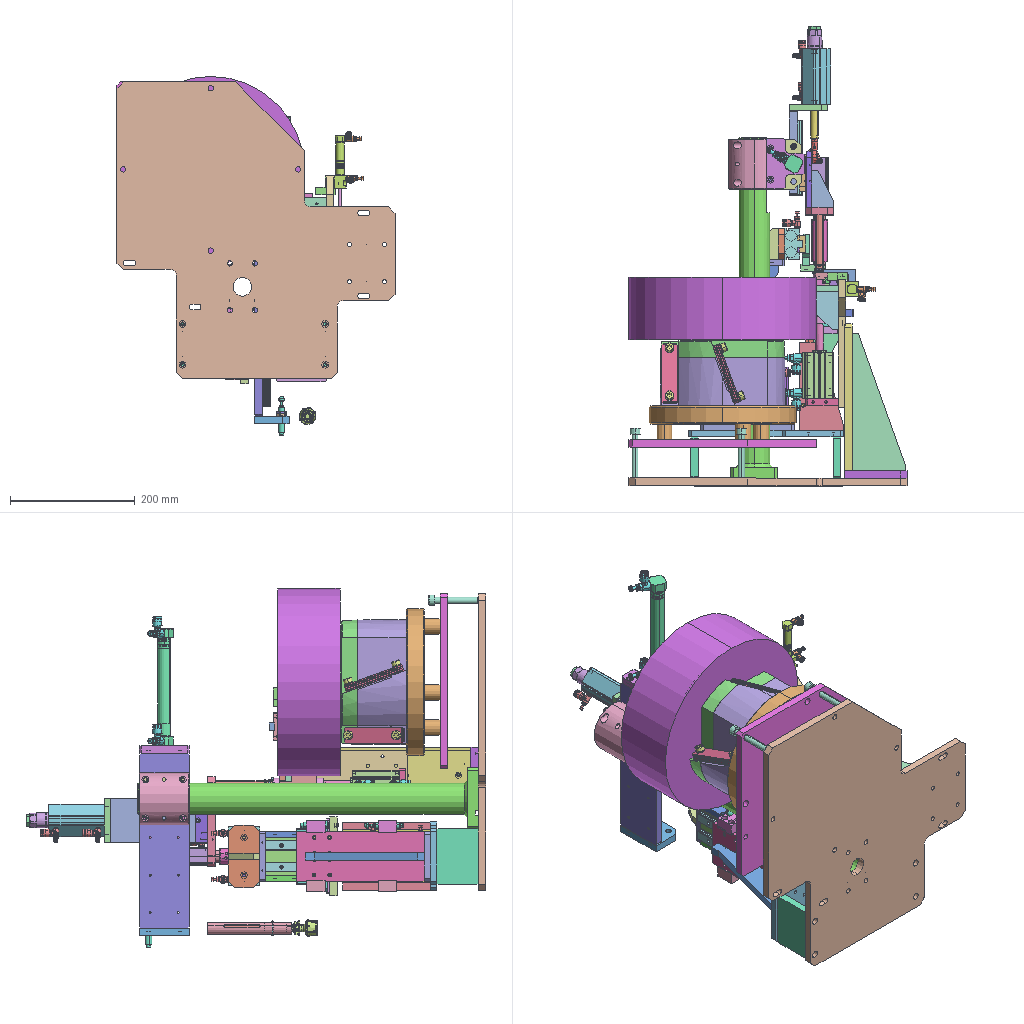Assembly | STEP file | 112 different items | 228 placed | box 445 x 736 x 575 mm
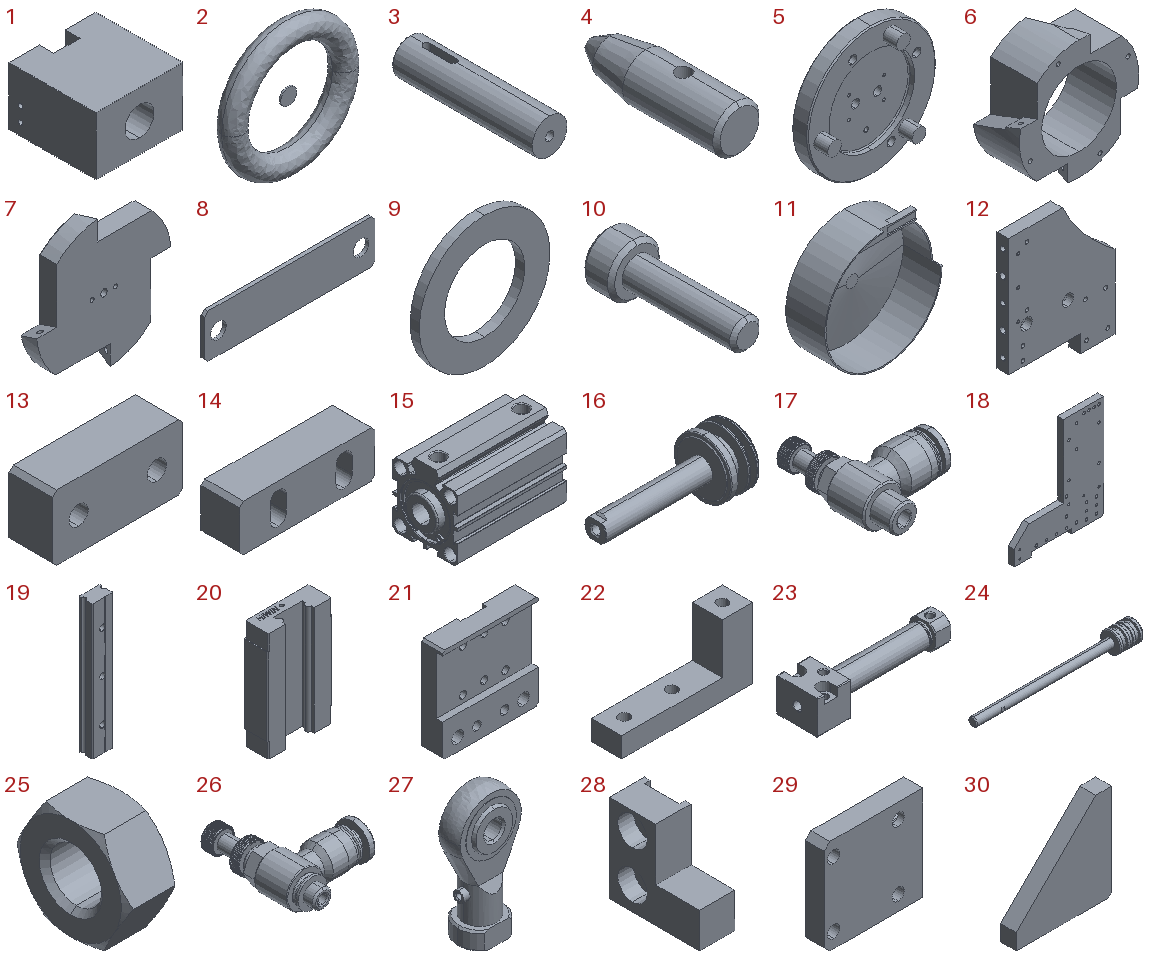Parts list (item | name | quantity | parent item | size | volume):
1 | PN_0053 | x1 | in PN_0052 | 60 x 60 x 40 mm | 121912 mm3
2 | 20501 | x14 | in PN_0052, PN_0061 | 16.4 x 2.7 x 16.4 mm | 247.033 mm3
3 | PN_0054 | x1 | in PN_0052 | 20 x 80 x 20 mm | 15788 mm3
4 | PN_0055 | x1 | in PN_0052 | 12.5 x 40 x 12.5 mm | 3984 mm3
5 | Vibration plate 3-04_default | x1 | in Vibration plate 3-02_default | 235 x 74 x 235 mm | 1320823 mm3
6 | Vibration plate 3-03_default | x1 | in Vibration plate 3-02_default | 200 x 78 x 200 mm | 1058700 mm3
7 | Vibration plate 3-08_default | x2 | in Vibration plate 3-02_default | 199.095 x 28 x 199.095 mm | 629211 mm3
8 | Vibration plate 3-07_default | x16 | in Vibration plate 3-02_default | 98 x 2 x 25 mm | 4630 mm3
9 | Vibration plate 3-06_default | x32 | in Vibration plate 3-02_default | 14 x 1 x 14 mm | 95.85 mm3
10 | Vibration plate 3-05_default | x12 | in Vibration plate 3-02_default | 14 x 38 x 14 mm | 2499 mm3
11 | Vibration plate 20501 | x1 | in Vibration plate 20501_default | 300 x 100 x 300 mm | 987568 mm3
12 | PN_0003 | x1 | in PN_0052 | 90 x 10 x 115 mm | 78081 mm3
13 | PN_0004 | x1 | in PN_0052 | 30 x 10 x 15 mm | 4176 mm3
14 | PN_0005 | x1 | in PN_0052 | 35 x 10 x 12 mm | 3567 mm3
15 | SDA32x40S-01-cc | x1 | in SDA32x40S-cc | 77.5 x 44 x 50 mm | 81433 mm3
16 | SDA32x40S-02-cc | x1 | in SDA32x40S-cc | 75.5 x 31.9 x 31.9 mm | 15906 mm3
17 | PSL801A | x4 | in SDA32x40S-cc, MI20x125SU-cc | 33.8 x 41.6 x 14.7 mm | 5385 mm3
18 | PN_0006 | x1 | in PN_0052 | 179.5 x 12 x 205 mm | 243420 mm3
19 | MGN12H-80-01-CC | x1 | in MGN12H-80-CC | 12 x 8 x 80 mm | 6824 mm3
20 | MGN12H-80-02-CC | x1 | in MGN12H-80-CC | 27 x 10 x 45.4 mm | 9266 mm3
21 | PN_0007 | x1 | in PN_0052 | 45 x 10 x 44.5 mm | 13324 mm3
22 | PN_0008 | x1 | in PN_0052 | 52 x 12 x 28 mm | 7462 mm3
23 | PBR12X30SU-01-CC | x1 | in PBR12X30SU-CC | 84 x 24.2 x 20 mm | 10911 mm3
24 | PBR12X30SU-02-CC | x1 | in PBR12X30SU-CC | 94.5 x 12 x 12 mm | 2851 mm3
25 | PBR12X30SU-03-CC | x1 | in PBR12X30SU-CC | 4 x 9.238 x 8 mm | 164.283 mm3
26 | PSL4M5A | x2 | in PBR12X30SU-CC | 23.8 x 30 x 9.8 mm | 1827 mm3
27 | F-M5X080U | x1 | in PBR12X30SU-CC | - | 2766 mm3
28 | PN_0009 | x1 | in PN_0052 | 12 x 31 x 30 mm | 6133 mm3
29 | PN_0010 | x1 | in PN_0052 | 52 x 10 x 50 mm | 23516 mm3
30 | PN_0011 | x1 | in PN_0052 | 60 x 10 x 60 mm | 22770 mm3
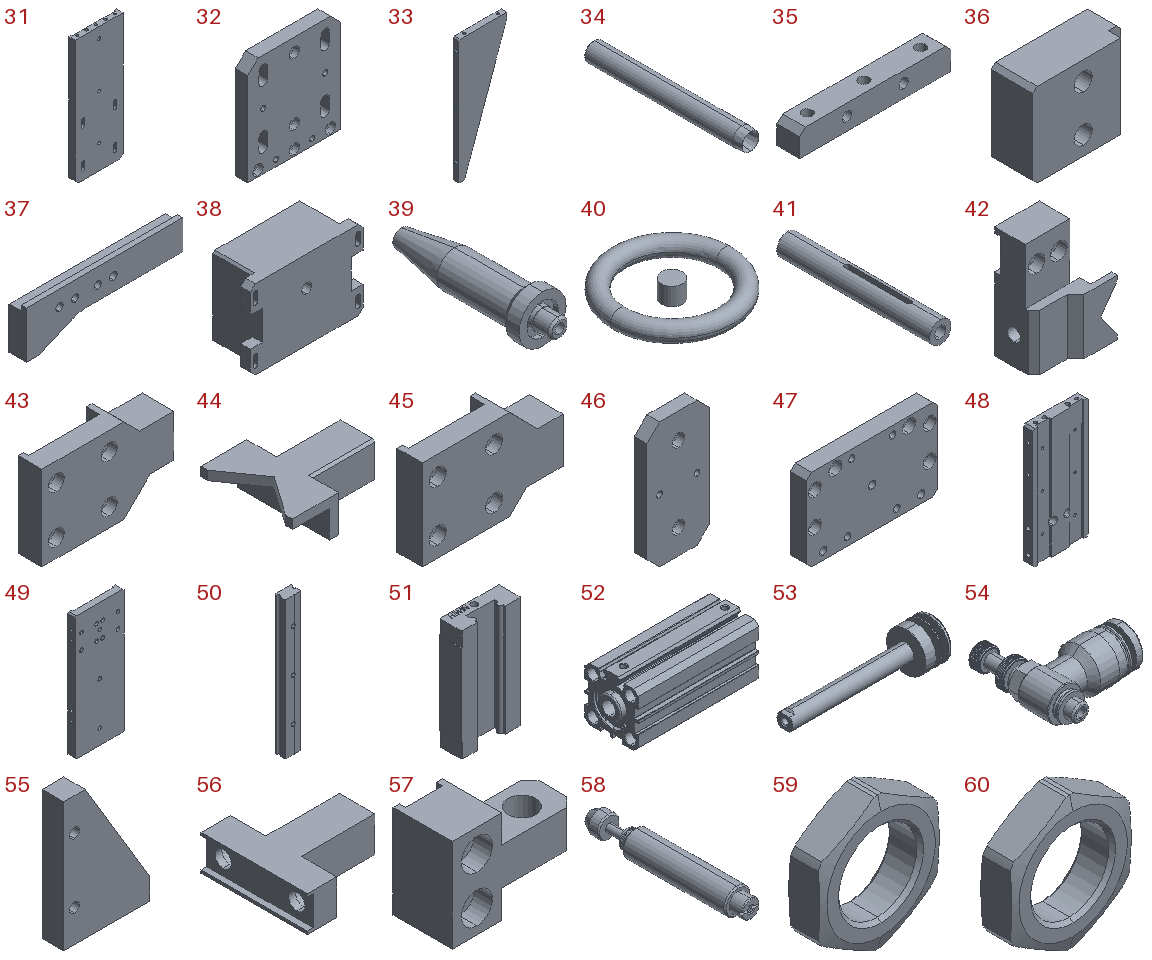31 | PN_0056 | x1 | in PN_0052 | 90 x 12 x 235.5 mm | 209838 mm3
32 | PN_0012 | x1 | in PN_0052 | 90 x 12 x 100 mm | 96261 mm3
33 | PN_0057 | x1 | in PN_0052 | 85 x 10 x 220 mm | 107342 mm3
34 | PN_0058 | x5 | in PN_0052, PN_0061, PN_0066 | 12.5 x 105 x 12.5 mm | 10895 mm3
35 | PN_0013 | x1 | in PN_0052 | 80 x 12 x 13 mm | 11040 mm3
36 | PN_0059 | x1 | in PN_0052 | 24 x 10 x 20 mm | 4313 mm3
37 | PN_0060 | x1 | in PN_0052 | 90 x 10 x 27 mm | 14739 mm3
38 | PN_0014 | x1 | in PN_0061 | 114 x 50 x 80 mm | 145177 mm3
39 | PN_0062 | x1 | in PN_0061 | 25 x 84 x 25 mm | 19612 mm3
40 | O-ring 11 diameter after expansion | x3 | in PN_0061, PN_0066 | 17.5 x 17.5 x 2.5 mm | 248.99 mm3
41 | PN_0063 | x3 | in PN_0061, PN_0066 | 19 x 135 x 19 mm | 21830 mm3
42 | PN_0015 | x1 | in PN_0061 | 27 x 17 x 40 mm | 6793 mm3
43 | PN_0016 | x1 | in PN_0061 | 50 x 12 x 32 mm | 11255 mm3
44 | PN_0017 | x2 | in PN_0061 | 24 x 20 x 8 mm | 1291 mm3
45 | PN_0018 | x1 | in PN_0061 | 50 x 12 x 32 mm | 11255 mm3
46 | PN_0019 | x1 | in PN_0061 | 50 x 10 x 100 mm | 45504 mm3
47 | PN_0020 | x1 | in PN_0061 | 80 x 10 x 50 mm | 36297 mm3
48 | PN_0021 | x1 | in PN_0061 | 60 x 10 x 130 mm | 67558 mm3
49 | PN_0022 | x1 | in PN_0061 | 80 x 12 x 203.5 mm | 178921 mm3
50 | MGN15H-130-01-cc | x2 | in MGN15H-130-cc | 15 x 10 x 130 mm | 18038 mm3
51 | MGN15H-130-02-cc | x2 | in MGN15H-130-cc | 32 x 12 x 58.8 mm | 16948 mm3
52 | SDA25x60S-01-cc | x1 | in SDA25x60S-cc | 93 x 40 x 42 mm | 80745 mm3
53 | SDA25x60S-02-cc | x1 | in SDA25x60S-cc | 93 x 24.9 x 24.9 mm | 11912 mm3
54 | PSL6M5A | x8 | in SDA25x60S-cc, MHF2-16D1_32-CC, ACQJ25x50-10S-cc, ACQ16x50S-cc | 28.6 x 30 x 12.5 mm | 2559 mm3
55 | PN_0023 | x1 | in PN_0061 | 40 x 10 x 60 mm | 15663 mm3
56 | PN_0024 | x2 | in PN_0061 | 35 x 36 x 12 mm | 6195 mm3
57 | PN_0025 | x2 | in PN_0061 | 40 x 19 x 30 mm | 10416 mm3
58 | ACA1007-01 | x4 | in ACA1007-cc | 10 x 62 x 10 mm | 3798 mm3
59 | ACA1007-02 | x4 | in ACA1007-cc | 14 x 4 x 15.686 mm | 394.069 mm3
60 | ACA1007-03 | x4 | in ACA1007-cc | 14 x 4 x 15.686 mm | 394.069 mm3
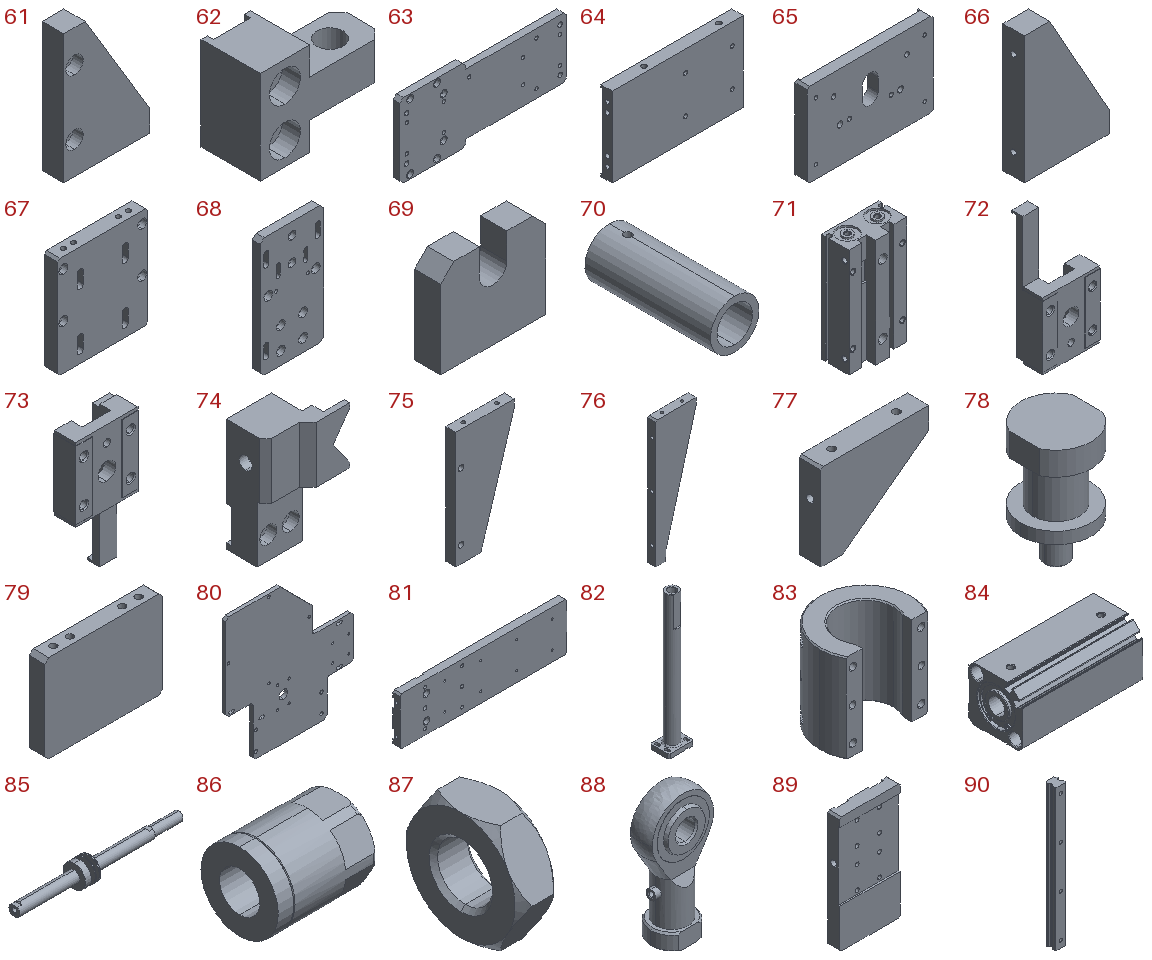61 | PN_0026 | x1 | in PN_0061 | 40 x 10 x 60 mm | 15663 mm3
62 | PN_0027 | x2 | in PN_0061 | 40 x 19 x 30 mm | 10499 mm3
63 | PN_0028 | x1 | in PN_0061 | 248 x 10 x 110 mm | 235264 mm3
64 | PN_0029 | x1 | in PN_0061 | 140 x 12 x 85 mm | 117738 mm3
65 | PN_0030 | x1 | in PN_0061 | 120 x 12 x 80 mm | 90970 mm3
66 | PN_0031 | x2 | in PN_0061 | 40 x 10 x 60 mm | 16813 mm3
67 | PN_0032 | x1 | in PN_0061 | 80 x 12 x 90 mm | 80517 mm3
68 | PN_0037 | x1 | in PN_0061 | 80 x 10 x 150 mm | 108687 mm3
69 | PN_0038 | x1 | in PN_0061 | 40 x 10 x 35 mm | 12065 mm3
70 | PN_0064 | x2 | in PN_0061, PN_0066 | 26 x 67 x 26 mm | 16488 mm3
71 | MHF2-16D1_32-01-CC | x1 | in MHF2-16D1_32-CC | 50 x 28.3 x 94 mm | 105067 mm3
72 | MHF2-16D1_32-02-CC | x1 | in MHF2-16D1_32-CC | 27 x 14.6 x 60.3 mm | 7195 mm3
73 | MHF2-16D1_32-03-CC | x1 | in MHF2-16D1_32-CC | 27 x 14.6 x 60.3 mm | 7195 mm3
74 | PN_0039 | x1 | in PN_0061 | 27 x 17 x 40 mm | 6793 mm3
75 | PN_0033 | x2 | in PN_0061 | 70 x 12 x 140 mm | 85204 mm3
76 | PN_0034 | x1 | in PN_0061 | 60 x 12 x 190 mm | 83127 mm3
77 | PN_0035 | x1 | in PN_0061 | 50 x 10 x 40 mm | 13691 mm3
78 | PN_0036 | x1 | in PN_0061 | 15 x 15 x 25.5 mm | 2226 mm3
79 | PN_0065 | x2 | in PN_0061 | 90 x 12 x 67 mm | 69945 mm3
80 | PN_0001 | x1 | - | 445 x 12 x 475 mm | 1746593 mm3
81 | PN_0040 | x1 | in PN_0066 | 280 x 12 x 80 mm | 245567 mm3
82 | PN_0041 | x1 | in PN_0066 | 100 x 75 x 545 mm | 756375 mm3
83 | PN_0042 | x1 | in PN_0066 | 83 x 61 x 80 mm | 174767 mm3
84 | ACQJ25x50-10S-01-cc | x1 | in ACQJ25x50-10S-cc | 89 x 40 x 40 mm | 88799 mm3
85 | ACQJ25x50-10S-02-cc | x1 | in ACQJ25x50-10S-cc | 180.5 x 25 x 25 mm | 23193 mm3
86 | ACQJ25x50-10S-03-cc | x1 | in ACQJ25x50-10S-cc | 31 x 24 x 24 mm | 10448 mm3
87 | ACQJ25x50-10S-04-cc | x1 | in ACQJ25x50-10S-cc | 6 x 19.63 x 17 mm | 1118 mm3
88 | F-M6X100U | x1 | in ACQJ25x50-10S-cc | - | 3624 mm3
89 | PN_0043 | x1 | in PN_0066 | 70 x 14 x 135 mm | 108466 mm3
90 | HGH15CA-230-01 | x2 | in HGH15CA-230 | 15 x 15 x 200 mm | 36597 mm3
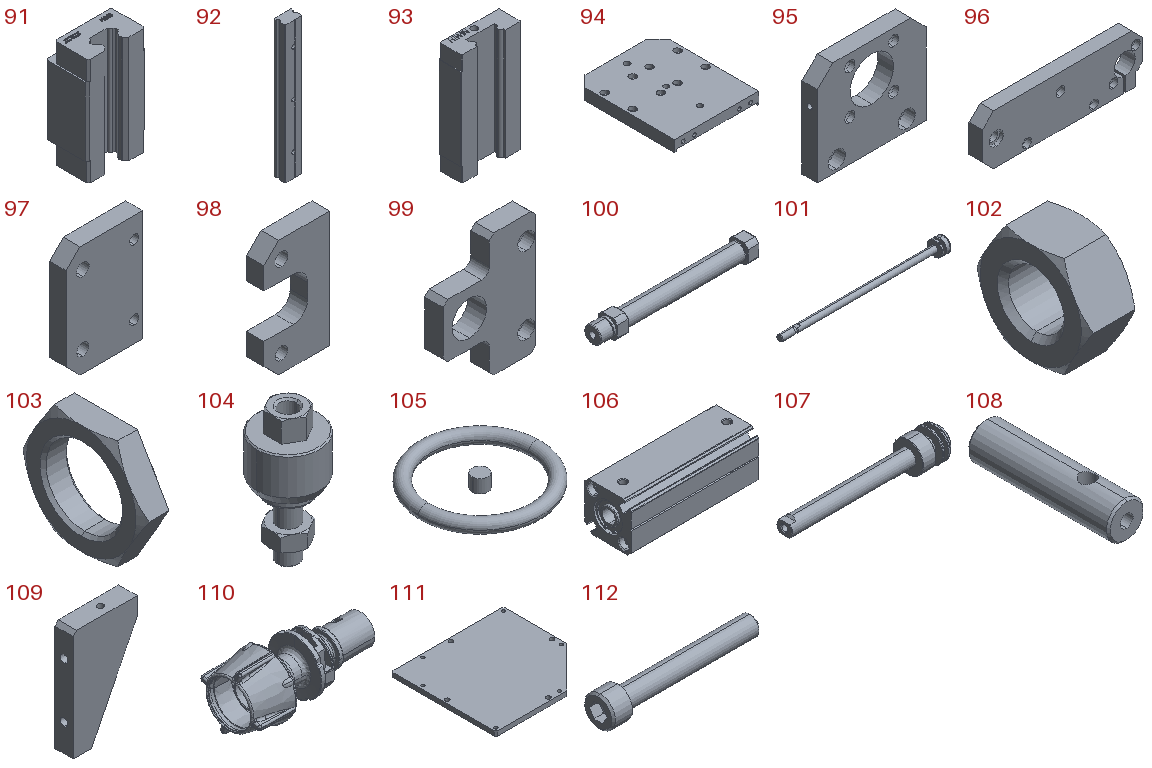91 | HGH15CA-230-02 | x2 | in HGH15CA-230 | 34 x 23.7 x 61.7 mm | 37046 mm3
92 | MGN15H-120-01 | x2 | in MGN15H-120 | 15 x 10 x 120 mm | 16613 mm3
93 | MGN15H-120-02 | x2 | in MGN15H-120 | 32 x 12 x 58.8 mm | 16948 mm3
94 | PN_0044 | x1 | in PN_0066 | 75 x 90 x 10 mm | 51506 mm3
95 | PN_0045 | x1 | in PN_0066 | 70 x 10 x 62 mm | 31607 mm3
96 | PN_0046 | x1 | in PN_0066 | 144 x 12 x 45 mm | 67965 mm3
97 | PN_0047 | x1 | in PN_0066 | 55 x 12 x 80 mm | 48507 mm3
98 | PN_0048 | x1 | in PN_0066 | 45 x 12 x 80 mm | 29583 mm3
99 | PN_0049 | x1 | in PN_0066 | 60 x 12 x 80 mm | 34785 mm3
100 | MI20x125SU-01-cc | x1 | in MI20x125SU-cc | 207 x 25 x 25 mm | 36262 mm3
101 | MI20x125SU-02-cc | x1 | in MI20x125SU-cc | 216.2 x 19.5 x 19.5 mm | 13209 mm3
102 | MI20x125SU-03-cc | x1 | in MI20x125SU-cc | 6 x 13.856 x 12 mm | 526.038 mm3
103 | MI20x125SU-04-cc | x1 | in MI20x125SU-cc | 7 x 33.486 x 29 mm | 2690 mm3
104 | F-M8X125F | x1 | in MI20x125SU-cc | 24 x 24 x 51 mm | 10528 mm3
105 | O-ring 11 diameter after expansion 19 | x3 | in PN_0066 | 23.5 x 23.5 x 2.5 mm | 341.518 mm3
106 | ACQ16x50S-01-cc | x1 | in ACQ16x50S-cc | 80.5 x 29 x 29 mm | 45504 mm3
107 | ACQ16x50S-02-cc | x1 | in ACQ16x50S-cc | 80 x 16 x 16 mm | 5471 mm3
108 | PN_0050 | x1 | in PN_0066 | 9.5 x 36.5 x 9.5 mm | 2304 mm3
109 | PN_0051 | x1 | in PN_0066 | 35 x 10 x 60 mm | 14229 mm3
110 | Product1 | x1 | in PN_0066 | 57.85 x 26.867 x 26.867 mm | 9145 mm3
111 | PN_0002 | x1 | - | 300 x 280 x 12 mm | 926303 mm3
112 | CB10-70 | x2 | - | 80 x 16 x 16 mm | 7177 mm3
Placements (level | parent | child | x y z in mm | rotation matrix by rows):
1 | subassembly 2 | PN_0052 | -307.72 131.32 281.536 | 1 0 0 0 1 0 0 0 1
2 | PN_0052 | PN_0053 | -1.536 -12.972 30.0 | 1 0 0 0 1 0 0 0 1
2 | PN_0052 | 20501 | -1.536 42.928 30.0 | 0.606 0 0.7955 0 1 0 -0.7955 0 0.606
2 | PN_0052 | PN_0054 | -1.536 -42.972 30.0 | 0.01979 0 0.9998 0 1 0 -0.9998 0 0.01979
2 | PN_0052 | PN_0055 | -1.536 12.028 30.0 | 0.01979 0 0.9998 0 1 0 -0.9998 0 0.01979
2 | PN_0052 | 20501 | -1.536 34.787 30.0 | 0.7353 0 -0.6777 0 1 0 0.6777 0 0.7353
2 | PN_0052 | 20501 | 1.964 17.128 58.2 | -0.2944 0 0.9557 0 -1 0 0.9557 0 0.2944
2 | PN_0052 | Vibration plate 20501_default | -36.021 -209.789 155.625 | 1 0 0 0 0 -1 0 1 0
3 | Vibration plate 20501_default | Vibration plate 3-02_default | -238.015 155.671 -4.821 | 1 0 0 0 0 1 0 -1 0
4 | Vibration plate 3-02_default | Vibration plate 3-04_default | 117.5 -0.0041 -117.5 | 1 0 0 0 1 0 0 0 1
4 | Vibration plate 3-02_default | Vibration plate 3-03_default | 117.5 28.996 -117.5 | 1 0 0 0 1 0 0 0 1
4 | Vibration plate 3-02_default | Vibration plate 3-08_default | 117.5 106.996 -117.5 | 1 0 0 0 1 0 0 0 1
4 | Vibration plate 3-02_default | Vibration plate 3-08_default | 117.5 106.996 -117.5 | 1 0 0 0 1 0 0 0 1
4 | Vibration plate 3-02_default | Vibration plate 3-07_default | 202.5 78.474 -118.381 | 0 0 1 -0.9397 0.342 0 -0.342 -0.9397 0
4 | Vibration plate 3-02_default | Vibration plate 3-07_default | 202.5 79.5 -121.2 | 0 0 1 -0.9397 0.342 0 -0.342 -0.9397 0
4 | Vibration plate 3-02_default | Vibration plate 3-07_default | 202.5 80.526 -124.019 | 0 0 1 -0.9397 0.342 0 -0.342 -0.9397 0
4 | Vibration plate 3-02_default | Vibration plate 3-07_default | 202.5 81.552 -126.838 | 0 0 1 -0.9397 0.342 0 -0.342 -0.9397 0
4 | Vibration plate 3-02_default | Vibration plate 3-07_default | 116.619 78.474 -202.5 | -0.342 -0.9397 0 -0.9397 0.342 0 0 0 -1
4 | Vibration plate 3-02_default | Vibration plate 3-07_default | 113.8 79.5 -202.5 | -0.342 -0.9397 0 -0.9397 0.342 0 0 0 -1
4 | Vibration plate 3-02_default | Vibration plate 3-07_default | 110.981 80.526 -202.5 | -0.342 -0.9397 0 -0.9397 0.342 0 0 0 -1
4 | Vibration plate 3-02_default | Vibration plate 3-07_default | 108.162 81.552 -202.5 | -0.342 -0.9397 0 -0.9397 0.342 0 0 0 -1
4 | Vibration plate 3-02_default | Vibration plate 3-07_default | 32.5 78.474 -116.619 | 0 0 -1 -0.9397 0.342 0 0.342 0.9397 -0
4 | Vibration plate 3-02_default | Vibration plate 3-07_default | 32.5 79.5 -113.8 | 0 0 -1 -0.9397 0.342 0 0.342 0.9397 -0
4 | Vibration plate 3-02_default | Vibration plate 3-07_default | 32.5 80.526 -110.981 | 0 0 -1 -0.9397 0.342 0 0.342 0.9397 -0
4 | Vibration plate 3-02_default | Vibration plate 3-07_default | 32.5 81.552 -108.162 | 0 0 -1 -0.9397 0.342 0 0.342 0.9397 -0
4 | Vibration plate 3-02_default | Vibration plate 3-07_default | 118.381 78.474 -32.5 | 0.342 0.9397 0 -0.9397 0.342 0 0 0 1
4 | Vibration plate 3-02_default | Vibration plate 3-07_default | 121.2 79.5 -32.5 | 0.342 0.9397 0 -0.9397 0.342 0 0 0 1
4 | Vibration plate 3-02_default | Vibration plate 3-07_default | 124.019 80.526 -32.5 | 0.342 0.9397 0 -0.9397 0.342 0 0 0 1
4 | Vibration plate 3-02_default | Vibration plate 3-07_default | 126.838 81.552 -32.5 | 0.342 0.9397 0 -0.9397 0.342 0 0 0 1
4 | Vibration plate 3-02_default | Vibration plate 3-06_default | 115.635 121.106 -32.5 | -0.342 -0.9397 0 0.9397 -0.342 0 0 0 1
4 | Vibration plate 3-02_default | Vibration plate 3-06_default | 112.816 120.08 -32.5 | -0.342 -0.9397 0 0.9397 -0.342 0 0 0 1
4 | Vibration plate 3-02_default | Vibration plate 3-06_default | 109.996 119.054 -32.5 | -0.342 -0.9397 0 0.9397 -0.342 0 0 0 1
4 | Vibration plate 3-02_default | Vibration plate 3-06_default | 107.177 118.028 -32.5 | -0.342 -0.9397 0 0.9397 -0.342 0 0 0 1
4 | Vibration plate 3-02_default | Vibration plate 3-06_default | 202.5 121.106 -115.635 | 0 0 1 0.9397 -0.342 0 0.342 0.9397 0
4 | Vibration plate 3-02_default | Vibration plate 3-06_default | 202.5 120.08 -112.816 | 0 0 1 0.9397 -0.342 0 0.342 0.9397 0
4 | Vibration plate 3-02_default | Vibration plate 3-06_default | 202.5 119.054 -109.996 | 0 0 1 0.9397 -0.342 0 0.342 0.9397 0
4 | Vibration plate 3-02_default | Vibration plate 3-06_default | 202.5 118.028 -107.177 | 0 0 1 0.9397 -0.342 0 0.342 0.9397 0
4 | Vibration plate 3-02_default | Vibration plate 3-06_default | 119.365 121.106 -202.5 | 0.342 0.9397 0 0.9397 -0.342 0 0 0 -1
4 | Vibration plate 3-02_default | Vibration plate 3-06_default | 122.185 120.08 -202.5 | 0.342 0.9397 0 0.9397 -0.342 0 0 0 -1
4 | Vibration plate 3-02_default | Vibration plate 3-06_default | 125.004 119.054 -202.5 | 0.342 0.9397 0 0.9397 -0.342 0 0 0 -1
4 | Vibration plate 3-02_default | Vibration plate 3-06_default | 127.823 118.028 -202.5 | 0.342 0.9397 0 0.9397 -0.342 0 0 0 -1
4 | Vibration plate 3-02_default | Vibration plate 3-06_default | 32.5 121.106 -119.365 | 0 0 -1 0.9397 -0.342 0 -0.342 -0.9397 -0
4 | Vibration plate 3-02_default | Vibration plate 3-06_default | 32.5 120.08 -122.185 | 0 0 -1 0.9397 -0.342 0 -0.342 -0.9397 -0
4 | Vibration plate 3-02_default | Vibration plate 3-06_default | 32.5 119.054 -125.004 | 0 0 -1 0.9397 -0.342 0 -0.342 -0.9397 -0
4 | Vibration plate 3-02_default | Vibration plate 3-06_default | 32.5 118.028 -127.823 | 0 0 -1 0.9397 -0.342 0 -0.342 -0.9397 -0
4 | Vibration plate 3-02_default | Vibration plate 3-06_default | 143.68 44.051 -32.5 | -0.342 -0.9397 0 0.9397 -0.342 0 0 0 1
4 | Vibration plate 3-02_default | Vibration plate 3-06_default | 140.861 43.025 -32.5 | -0.342 -0.9397 0 0.9397 -0.342 0 0 0 1
4 | Vibration plate 3-02_default | Vibration plate 3-06_default | 138.042 41.999 -32.5 | -0.342 -0.9397 0 0.9397 -0.342 0 0 0 1
4 | Vibration plate 3-02_default | Vibration plate 3-06_default | 135.223 40.973 -32.5 | -0.342 -0.9397 0 0.9397 -0.342 0 0 0 1
4 | Vibration plate 3-02_default | Vibration plate 3-06_default | 202.5 44.051 -143.68 | 0 0 1 0.9397 -0.342 0 0.342 0.9397 0
4 | Vibration plate 3-02_default | Vibration plate 3-06_default | 202.5 43.025 -140.861 | 0 0 1 0.9397 -0.342 0 0.342 0.9397 0
4 | Vibration plate 3-02_default | Vibration plate 3-06_default | 202.5 41.999 -138.042 | 0 0 1 0.9397 -0.342 0 0.342 0.9397 0
4 | Vibration plate 3-02_default | Vibration plate 3-06_default | 202.5 40.973 -135.223 | 0 0 1 0.9397 -0.342 0 0.342 0.9397 0
4 | Vibration plate 3-02_default | Vibration plate 3-06_default | 91.32 44.051 -202.5 | 0.342 0.9397 0 0.9397 -0.342 0 0 0 -1
4 | Vibration plate 3-02_default | Vibration plate 3-06_default | 94.139 43.025 -202.5 | 0.342 0.9397 0 0.9397 -0.342 0 0 0 -1
4 | Vibration plate 3-02_default | Vibration plate 3-06_default | 96.958 41.999 -202.5 | 0.342 0.9397 0 0.9397 -0.342 0 0 0 -1
4 | Vibration plate 3-02_default | Vibration plate 3-06_default | 99.777 40.973 -202.5 | 0.342 0.9397 0 0.9397 -0.342 0 0 0 -1
4 | Vibration plate 3-02_default | Vibration plate 3-06_default | 32.5 44.051 -91.32 | 0 0 -1 0.9397 -0.342 0 -0.342 -0.9397 -0
4 | Vibration plate 3-02_default | Vibration plate 3-06_default | 32.5 43.025 -94.139 | 0 0 -1 0.9397 -0.342 0 -0.342 -0.9397 -0
4 | Vibration plate 3-02_default | Vibration plate 3-06_default | 32.5 41.999 -96.958 | 0 0 -1 0.9397 -0.342 0 -0.342 -0.9397 -0
4 | Vibration plate 3-02_default | Vibration plate 3-06_default | 32.5 40.973 -99.777 | 0 0 -1 0.9397 -0.342 0 -0.342 -0.9397 -0
4 | Vibration plate 3-02_default | Vibration plate 3-05_default | 32.5 110.845 -147.556 | 0 0 1 0.9397 0.342 0 -0.342 0.9397 0
4 | Vibration plate 3-02_default | Vibration plate 3-05_default | 32.5 33.79 -119.511 | 0 0 1 0.9397 0.342 0 -0.342 0.9397 0
4 | Vibration plate 3-02_default | Vibration plate 3-05_default | 87.444 110.845 -32.5 | -0.342 0.9397 0 0.9397 0.342 0 0 0 -1
4 | Vibration plate 3-02_default | Vibration plate 3-05_default | 115.49 33.79 -32.5 | -0.342 0.9397 0 0.9397 0.342 0 0 0 -1
4 | Vibration plate 3-02_default | Vibration plate 3-05_default | 202.5 110.845 -87.444 | 0 0 -1 0.9397 0.342 0 0.342 -0.9397 -0
4 | Vibration plate 3-02_default | Vibration plate 3-05_default | 202.5 33.79 -115.49 | 0 0 -1 0.9397 0.342 0 0.342 -0.9397 -0
4 | Vibration plate 3-02_default | Vibration plate 3-05_default | 147.556 110.845 -202.5 | 0.342 -0.9397 0 0.9397 0.342 0 0 0 1
4 | Vibration plate 3-02_default | Vibration plate 3-05_default | 119.511 33.79 -202.5 | 0.342 -0.9397 0 0.9397 0.342 0 0 0 1
4 | Vibration plate 3-02_default | Vibration plate 3-05_default | 199.5 38.996 -82.5 | -1 0 0 0 -1 0 0 0 1
4 | Vibration plate 3-02_default | Vibration plate 3-05_default | 82.5 38.996 -35.5 | 0 0 -1 0 -1 0 -1 0 -0
4 | Vibration plate 3-02_default | Vibration plate 3-05_default | 35.5 38.996 -152.5 | 1 0 0 0 -1 0 0 0 -1
4 | Vibration plate 3-02_default | Vibration plate 3-05_default | 152.5 38.996 -199.5 | 0 0 1 0 -1 0 1 0 0
3 | Vibration plate 20501_default | Vibration plate 20501 | -120.515 38.171 -239.817 | 1 0 0 0 0 -1 0 1 -0
2 | PN_0052 | PN_0003 | -16.536 17.028 100.0 | -1 0 0 0 -1 0 0 0 1
2 | PN_0052 | PN_0004 | -46.536 27.028 42.5 | -1 0 0 0 -1 0 0 0 1
2 | PN_0052 | PN_0005 | -44.036 27.028 73.0 | -1 0 0 0 -1 0 0 0 1
2 | PN_0052 | SDA32x40S-cc | -18.981 -89.972 29.214 | 0 0 -1 -1 0 0 0 1 0
3 | SDA32x40S-cc | SDA32x40S-01-cc | -0.0 0.7864 -17.446 | 1 0 0 0 1 0 0 0 1
3 | SDA32x40S-cc | SDA32x40S-02-cc | -40.0 0.7864 -17.446 | 1 0 0 0 -1 0.000992 0 -0.000992 -1
3 | SDA32x40S-cc | PSL801A | 9.0 0.7864 19.754 | 1 0 0 0 0 -1 0 1 0
3 | SDA32x40S-cc | PSL801A | 65.5 0.7864 19.754 | 1 0 0 0 0 -1 0 1 0
2 | PN_0052 | 20501 | -15.036 17.128 58.2 | -0.2944 0 0.9557 0 -1 0 0.9557 0 0.2944
2 | PN_0052 | 20501 | -32.036 17.128 58.2 | -0.2944 0 0.9557 0 -1 0 0.9557 0 0.2944
2 | PN_0052 | 20501 | -49.036 17.128 58.2 | -0.2944 0 0.9557 0 -1 0 0.9557 0 0.2944
2 | PN_0052 | 20501 | -66.036 17.128 58.2 | -0.2944 0 0.9557 0 -1 0 0.9557 0 0.2944
2 | PN_0052 | 20501 | -83.036 17.128 58.2 | -0.2944 0 0.9557 0 -1 0 0.9557 0 0.2944
2 | PN_0052 | 20501 | -100.036 17.128 58.2 | -0.2944 0 0.9557 0 -1 0 0.9557 0 0.2944
2 | PN_0052 | PN_0006 | 28.464 -90.472 77.5 | 0 1 0 0 0 -1 -1 0 0
2 | PN_0052 | MGN12H-80-CC | 68.74 20.968 40 | 1 0 0 0 1 0 0 0 1
3 | MGN12H-80-CC | MGN12H-80-01-CC | -48.275 -3.941 70 | 1 0 0 0 1 0 0 0 1
3 | MGN12H-80-CC | MGN12H-80-02-CC | -48.275 -3.941 82.5 | 1 0 0 0 1 0 0 0 1
2 | PN_0052 | PN_0007 | 13.714 27.028 122.5 | 0 0 1 0 1 0 -1 0 -0
2 | PN_0052 | PN_0008 | 44.464 35.028 116.5 | 1 0 0 0 0 -1 0 1 0
2 | PN_0052 | PBR12X30SU-CC | 50.464 10.928 165.0 | 0 0 1 0 -1 0 1 0 -0
3 | PBR12X30SU-CC | PBR12X30SU-01-CC | -0.0 -0.0 -0.0 | 1 0 0 0 1 0 0 0 1
3 | PBR12X30SU-CC | PBR12X30SU-02-CC | -30.0 -0.0 -0.0 | 1 0 0 0 -0.9328 0.3605 0 -0.3605 -0.9328
3 | PBR12X30SU-CC | PBR12X30SU-03-CC | -30.5 -0.0 0.0 | 1 0 0 0 -0.9237 0.383 0 -0.383 -0.9237
3 | PBR12X30SU-CC | PSL4M5A | 15.5 0.0 16.7 | -0.1859 0 0.9826 0.9826 0 0.1859 0 1 0
3 | PBR12X30SU-CC | F-M5X080U | -43.0 -0.0 -0.0 | 0 0 -1 0 -1 0 -1 0 0
3 | PBR12X30SU-CC | PSL4M5A | 79.0 0.0 14.2 | 0.3802 0 0.9249 0.9249 0 -0.3802 0 1 0
2 | PN_0052 | PN_0009 | 26.464 31.028 169.5 | 0 1 0 -1 0 0 0 0 1
2 | PN_0052 | PN_0010 | 2.464 -164.472 30.0 | 1 0 0 0 -1 0 0 0 -1
2 | PN_0052 | PN_0011 | -1.536 -22.972 85.0 | 0 0 -1 1 0 0 0 -1 0
2 | PN_0052 | PN_0056 | 50.464 -161.722 45.0 | 0 -1 0 0 0 -1 1 0 0
2 | PN_0052 | PN_0012 | 88.464 -291.472 45.0 | 0 0 1 0 1 0 -1 0 0
2 | PN_0052 | PN_0057 | 92.964 -169.472 40.0 | 1 0 0 0 0 -1 0 1 0
2 | PN_0052 | PN_0058 | -1.536 28.028 30.0 | -0.7289 0 0.6846 0 1 0 -0.6846 0 -0.7289
2 | PN_0052 | PN_0058 | -1.536 28.028 -85.0 | -0.7289 0 0.6846 0 1 0 -0.6846 0 -0.7289
2 | PN_0052 | PN_0058 | -1.536 28.028 -200.0 | -0.7289 0 0.6846 0 1 0 -0.6846 0 -0.7289
2 | PN_0052 | 20501 | -1.536 50.128 30.0 | -0.2248 0 0.9744 0 -1 0 0.9744 0 0.2248
2 | PN_0052 | 20501 | -1.536 50.128 -85.0 | -0.2248 0 0.9744 0 -1 0 0.9744 0 0.2248
2 | PN_0052 | 20501 | -1.536 50.128 -200.0 | -0.2248 0 0.9744 0 -1 0 0.9744 0 0.2248
2 | PN_0052 | PN_0013 | 46.964 -32.972 45.0 | 0 0 1 0 1 0 -1 0 0
2 | PN_0052 | PN_0059 | 16.464 17.028 60.0 | -1 0 0 0 1 0 0 0 -1
2 | PN_0052 | PN_0060 | -2.036 17.028 97.0 | 0 0 1 0 1 0 -1 0 -0
1 | subassembly 2 | PN_0061 | -389.256 99.671 182.689 | 0 0 1 0 1 0 -1 0 0
2 | PN_0061 | PN_0014 | -13.847 -18.68 70.0 | 1 0 0 0 1 0 0 0 1
2 | PN_0061 | PN_0062 | -13.847 -8.68 80.0 | -0.7709 0 0.637 0 1 0 -0.637 0 -0.7709
2 | PN_0061 | 20501 | -13.847 59.72 80.0 | 0.9776 0 -0.2103 0 1 0 0.2103 0 0.9776
2 | PN_0061 | PN_0058 | -13.847 60.082 80.0 | -0.9919 0 -0.1266 0 1 0 0.1266 0 -0.9919
2 | PN_0061 | O-ring 11 diameter after expansion | 19.903 30.446 26.253 | 0.9233 -0.3841 -0.004328 -0.006874 -0.02779 0.9996 -0.3841 -0.9229 -0.02829
2 | PN_0061 | O-ring 11 diameter after expansion | -13.847 49.349 80.0 | 0.3911 -0.9204 0 0 0 1 -0.9204 -0.3911 0
2 | PN_0061 | PN_0063 | -13.847 174.382 80.0 | -0.9978 0 -0.06595 0 -1 0 -0.06595 0 0.9978
2 | PN_0061 | PN_0015 | 7.997 65.875 80.0 | -1 0 0 0 1 0 0 0 -1
2 | PN_0061 | PN_0016 | 11.497 105.875 64.0 | 0 0 1 -1 0 0 0 -1 0
2 | PN_0061 | PN_0017 | -33.69 75.875 90.0 | -1 0 0 0 0 -1 0 -1 -0
2 | PN_0061 | PN_0017 | 6.497 75.875 70.0 | 1 0 0 0 0 -1 0 1 0
2 | PN_0061 | PN_0018 | -39.19 105.875 64.0 | 0 0 1 -1 0 0 0 -1 -0
2 | PN_0061 | PN_0019 | -13.847 115.375 14.0 | 0 0 -1 -1 0 0 0 1 0
2 | PN_0061 | PN_0020 | -13.847 90.375 -1.0 | 1 0 0 0 -1 0 0 0 -1
2 | PN_0061 | PN_0021 | -13.847 15.375 -26.0 | -1 0 0 0 0 1 0 1 0
2 | PN_0061 | PN_0022 | -13.847 -71.073 -50.0 | -1 0 0 0 0 1 0 1 0
2 | PN_0061 | MGN15H-130-cc | -16.654 125.375 -30.34 | -1 0 0 0 0 -1 0 -1 -0
3 | MGN15H-130-cc | MGN15H-130-01-cc | -20.307 -6.34 110 | 1 0 0 0 1 0 0 0 1
3 | MGN15H-130-cc | MGN15H-130-02-cc | -20.308 -6.34 124.699 | 1 0 0 0 1 0 0 0 1
2 | PN_0061 | MGN15H-130-cc | -51.654 125.375 -30.34 | -1 0 0 0 0 -1 0 -1 -0
3 | MGN15H-130-cc | MGN15H-130-01-cc | -20.307 -6.34 110 | 1 0 0 0 1 0 0 0 1
3 | MGN15H-130-cc | MGN15H-130-02-cc | -20.307 -6.34 124.699 | 1 0 0 0 1 0 0 0 1
2 | PN_0061 | SDA25x60S-cc | -13.847 18.677 10.0 | 0 0 -1 -1 0 0 0 1 0
3 | SDA25x60S-cc | SDA25x60S-01-cc | 100.5 -0.0 -0.0 | 1 0 0 0 1 0 0 0 1
3 | SDA25x60S-cc | SDA25x60S-02-cc | 48.801 -0.0 -0.0 | 1 0 0 0 0.309 -0.9511 0 0.9511 0.309
3 | SDA25x60S-cc | PSL6M5A | 186.0 0.0 30.5 | -0.001298 0 1 1 0 0.001298 0 1 0
3 | SDA25x60S-cc | PSL6M5A | 109.7 -0.433 30.5 | -0.001298 0 1 1 0 0.001298 0 1 0
2 | PN_0061 | PN_0023 | -43.847 80.375 -26.0 | 0 -1 0 0 0 -1 1 0 0
2 | PN_0061 | PN_0024 | -64.347 -33.625 -21.0 | -1 0 0 0 1 0 0 0 -1
2 | PN_0061 | PN_0025 | -70.847 0.6765 -44.0 | 0 1 0 0 0 1 1 0 0
2 | PN_0061 | PN_0025 | -70.847 -114.323 -44.0 | 0 1 0 0 0 1 1 0 0
2 | PN_0061 | ACA1007-cc | -63.347 -139.323 -22.0 | 0.9849 0 0.1733 0 1 0 -0.1733 0 0.9849
3 | ACA1007-cc | ACA1007-01 | 0.0 -0.0 -0.0 | 1 0 0 0 1 0 0 0 1
3 | ACA1007-cc | ACA1007-02 | 0.0 -0.0 -0.0 | 1 0 0 0 1 0 0 0 1
3 | ACA1007-cc | ACA1007-03 | 0.0 -0.0 -0.0 | 1 0 0 0 1 0 0 0 1
2 | PN_0061 | ACA1007-cc | -63.347 25.677 -22.0 | 0.9385 0 0.3452 0 -1 0 0.3452 0 -0.9385
3 | ACA1007-cc | ACA1007-01 | 0.0 -0.0 -0.0 | 1 0 0 0 1 0 0 0 1
3 | ACA1007-cc | ACA1007-02 | 0.0 -0.0 -0.0 | 1 0 0 0 1 0 0 0 1
3 | ACA1007-cc | ACA1007-03 | 0.0 -0.0 -0.0 | 1 0 0 0 1 0 0 0 1
2 | PN_0061 | PN_0026 | 26.153 80.375 -26.0 | 0 -1 0 0 0 -1 1 0 -0
2 | PN_0061 | PN_0027 | 43.153 0.6765 -44.0 | 0 -1 0 0 0 -1 1 0 -0
2 | PN_0061 | PN_0027 | 43.153 -114.323 -44.0 | 0 -1 0 0 0 -1 1 0 0
2 | PN_0061 | PN_0028 | -13.847 -192.823 -6.0 | 0 0 1 0 1 0 -1 0 -0
2 | PN_0061 | PN_0029 | -13.847 -112.823 48.0 | 0 0 1 1 0 0 0 1 0
2 | PN_0061 | PN_0030 | -13.847 -28.68 70.0 | 1 0 0 0 1 0 0 0 1
2 | PN_0061 | PN_0031 | 26.153 -58.68 90.0 | 0 -1 0 0 0 -1 1 0 0
2 | PN_0061 | PN_0031 | -43.847 -58.68 90.0 | 0 -1 0 0 0 -1 1 0 0
2 | PN_0061 | PN_0032 | -13.847 -73.68 58.0 | -1 0 0 0 0 1 0 1 0
2 | PN_0061 | PN_0037 | -13.847 -182.823 -35.0 | -1 0 0 0 1 0 0 0 -1
2 | PN_0061 | PN_0038 | -13.847 -21.625 1.5 | 1 0 0 0 1 0 0 0 1
2 | PN_0061 | PN_0064 | -13.847 87.382 80.0 | 0.9773 0 -0.2118 0 1 0 0.2118 0 0.9773
2 | PN_0061 | MHF2-16D1_32-CC | -8.793 122.417 22.196 | 0 0 1 -1 0 0 0 -1 -0
3 | MHF2-16D1_32-CC | MHF2-16D1_32-01-CC | 7.042 -1.804 -5.054 | 1 0 0 0 1 0 0 0 1
3 | MHF2-16D1_32-CC | MHF2-16D1_32-02-CC | 7.042 -1.804 1.303 | 1 0 0 0 1 0 0 0 1
3 | MHF2-16D1_32-CC | MHF2-16D1_32-03-CC | 7.042 -1.804 -11.41 | 1 0 0 0 1 0 0 0 1
3 | MHF2-16D1_32-CC | PSL6M5A | -26.458 -21.804 -42.054 | 0 -1 0 1 0 0 0 0 1
3 | MHF2-16D1_32-CC | PSL6M5A | -26.458 -21.804 31.946 | 0 -1 0 1 0 0 0 0 1
2 | PN_0061 | PN_0039 | -35.69 65.875 80.0 | 1 0 0 0 1 0 0 0 1
2 | PN_0061 | 20501 | -13.847 69.182 80.0 | 0.9776 0 -0.2103 0 1 0 0.2103 0 0.9776
2 | PN_0061 | PN_0024 | 36.653 -33.625 -21.0 | 1 0 0 0 1 0 0 0 1
2 | PN_0061 | PN_0033 | -56.347 -112.823 83.0 | 0 -1 0 0 0 -1 1 0 0
2 | PN_0061 | PN_0034 | -19.847 -77.823 -80.0 | 0 1 0 0 0 -1 -1 0 -0
2 | PN_0061 | PN_0033 | 40.653 -112.823 83.0 | 0 -1 0 0 0 -1 1 0 0
2 | PN_0061 | PN_0035 | -8.847 115.375 -6.0 | 0 -1 0 1 0 0 0 0 1
2 | PN_0061 | PN_0036 | -13.847 -21.625 10.0 | 1 0 0 0 0 1 0 -1 0
2 | PN_0061 | PN_0065 | -13.847 -259.824 108.0 | 1 0 0 0 0 1 0 -1 -0
2 | PN_0061 | PN_0065 | -13.847 -192.823 -120.0 | 1 0 0 0 0 -1 0 1 0
1 | subassembly 2 | PN_0001 | -391.756 -172.152 379.036 | 1 0 0 0 1 0 0 0 1
1 | subassembly 2 | PN_0066 | -227.853 468.659 19.652 | 0 1 0 0 0 -1 -1 0 0
2 | PN_0066 | PN_0040 | -201.883 -165.902 125.811 | 1 0 0 0 1 0 0 0 1
2 | PN_0066 | ACA1007-cc | -30.884 -122.902 100.811 | 0 -1 0 0.2349 0 -0.972 0.972 0 0.2349
3 | ACA1007-cc | ACA1007-01 | 0.0 -0.0 -0.0 | 1 0 0 0 1 0 0 0 1
3 | ACA1007-cc | ACA1007-02 | 0.0 -0.0 -0.0 | 1 0 0 0 1 0 0 0 1
3 | ACA1007-cc | ACA1007-03 | 0.0 -0.0 -0.0 | 1 0 0 0 1 0 0 0 1
2 | PN_0066 | PN_0041 | -247.383 352.098 1006.311 | 1 0 0 0 -1 0 0 0 -1
2 | PN_0066 | PN_0042 | -290.384 352.098 -496.189 | -1 0 0 0 -1 0 0 0 1
2 | PN_0066 | ACQJ25x50-10S-cc | -234.383 -89.402 30.311 | 0 0.7071 0.7071 0 0.7071 -0.7071 -1 0 0
3 | ACQJ25x50-10S-cc | ACQJ25x50-10S-01-cc | -0.0 -0.0 -0.0 | 1 0 0 0 1 0 0 0 1
3 | ACQJ25x50-10S-cc | ACQJ25x50-10S-02-cc | -50.0 0.0 0.0 | 1 0 0 0 -0.9327 0.3606 0 -0.3606 -0.9327
3 | ACQJ25x50-10S-cc | ACQJ25x50-10S-03-cc | -50.0 -0.0 -0.0 | 1 0 0 0 1 0 0 0 1
3 | ACQJ25x50-10S-cc | ACQJ25x50-10S-04-cc | -50.0 -0.0 -0.0 | 1 0 0 0 1 0 0 0 1
3 | ACQJ25x50-10S-cc | F-M6X100U | -55.0 -0.0 -0.0 | 0 0 -1 0.7071 0.7071 0 0.7071 -0.7071 -0
3 | ACQJ25x50-10S-cc | PSL6M5A | 11.0 -0.0 28.5 | 1 0 0 0 0 -1 0 1 0
3 | ACQJ25x50-10S-cc | PSL6M5A | 78.0 -0.0 28.5 | 1 0 0 0 0 -1 0 1 0
2 | PN_0066 | PN_0043 | -234.383 -129.902 107.811 | 1 0 0 0 1 0 0 0 1
2 | PN_0066 | HGH15CA-230 | -206.883 -140.902 103.311 | 0 0 1 0 1 0 -1 0 0
3 | HGH15CA-230 | HGH15CA-230-01 | -0.0 -0.0 -0.0 | 1 0 0 0 1 0 0 0 1
3 | HGH15CA-230 | HGH15CA-230-02 | -0.0 -0.0 -27.5 | 1 0 0 0 1 0 0 0 1
2 | PN_0066 | HGH15CA-230 | -206.883 -140.902 148.311 | 0 0 1 0 1 0 -1 0 0
3 | HGH15CA-230 | HGH15CA-230-01 | -0.0 -0.0 -0.0 | 1 0 0 0 1 0 0 0 1
3 | HGH15CA-230 | HGH15CA-230-02 | -0.0 -0.0 -27.5 | 1 0 0 0 1 0 0 0 1
2 | PN_0066 | MGN15H-120 | -234.076 -111.562 5.311 | 1 0 0 0 1 0 0 0 1
3 | MGN15H-120 | MGN15H-120-01 | -20.307 -6.34 110 | 1 0 0 0 1 0 0 0 1
3 | MGN15H-120 | MGN15H-120-02 | -20.307 -6.34 135 | 1 0 0 0 1 0 0 0 1
2 | PN_0066 | MGN15H-120 | -194.076 -111.562 5.311 | 1 0 0 0 1 0 0 0 1
3 | MGN15H-120 | MGN15H-120-01 | -20.307 -6.34 110 | 1 0 0 0 1 0 0 0 1
3 | MGN15H-120 | MGN15H-120-02 | -20.307 -6.34 135 | 1 0 0 0 1 0 0 0 1
2 | PN_0066 | PN_0044 | -234.383 -103.902 150.311 | 1 0 0 0 0 1 0 -1 0
2 | PN_0066 | PN_0045 | -234.383 -98.902 30.311 | -1 0 0 0 0 1 0 1 0
2 | PN_0066 | PN_0046 | -234.383 -81.402 207.311 | 1 0 0 0 0 1 0 -1 0
2 | PN_0066 | PN_0047 | -61.883 -138.402 125.811 | 0 1 0 -1 0 0 0 0 1
2 | PN_0066 | PN_0048 | -303.884 -133.402 125.811 | 0 1 0 -1 0 0 0 0 1
2 | PN_0066 | PN_0049 | -353.884 -135.902 125.811 | 0 1 0 -1 0 0 0 0 1
2 | PN_0066 | MI20x125SU-cc | -353.884 -122.902 125.811 | -1 0 0 0 -0.8783 -0.4781 0 -0.4781 0.8783
3 | MI20x125SU-cc | MI20x125SU-01-cc | -0.0 -0.0 -0.0 | 1 0 0 0 1 0 0 0 1
3 | MI20x125SU-cc | MI20x125SU-02-cc | -4.5 0.0 0.0 | 1 0 0 0 0.5771 0.8167 0 -0.8167 0.5771
3 | MI20x125SU-cc | MI20x125SU-03-cc | -3.5 0.0 0.0 | 1 0 0 0 1 0 0 0 1
3 | MI20x125SU-cc | MI20x125SU-04-cc | -8.0 0.0 -0.0 | 1 0 0 0 1 0 0 0 1
3 | MI20x125SU-cc | PSL801A | 7.5 21.7 -0.0 | 0.9996 0 0.02858 0 1 0 -0.02858 0 0.9996
3 | MI20x125SU-cc | PSL801A | 179.5 21.7 -0.0 | 0.9996 0 0.02858 0 1 0 -0.02858 0 0.9996
3 | MI20x125SU-cc | F-M8X125F | -91.5 0.0 0.0 | 0 0 1 0 1 0 -1 0 0
2 | PN_0066 | ACA1007-cc | -322.884 -122.902 97.811 | 0 1 0 0.8086 0 0.5883 0.5883 0 -0.8086
3 | ACA1007-cc | ACA1007-01 | 0.0 -0.0 -0.0 | 1 0 0 0 1 0 0 0 1
3 | ACA1007-cc | ACA1007-02 | 0.0 -0.0 -0.0 | 1 0 0 0 1 0 0 0 1
3 | ACA1007-cc | ACA1007-03 | 0.0 -0.0 -0.0 | 1 0 0 0 1 0 0 0 1
2 | PN_0066 | PN_0058 | -291.884 -81.402 309.311 | 0.7387 0 -0.6741 0.6741 0 0.7387 0 -1 0
2 | PN_0066 | PN_0063 | -176.883 -81.402 195.311 | 0.9216 0 -0.3881 -0.3881 0 -0.9216 0 1 0
2 | PN_0066 | PN_0064 | -176.883 -81.402 282.311 | 0.9216 0 0.3881 -0.3881 0 0.9216 0 -1 0
2 | PN_0066 | PN_0063 | -61.883 -81.402 195.311 | 0.9216 0 -0.3881 -0.3881 0 -0.9216 0 1 0
2 | PN_0066 | O-ring 11 diameter after expansion 19 | -61.883 -81.402 299.061 | 0.9993 -0.03625 0 0.03625 0.9993 0 0 0 1
2 | PN_0066 | O-ring 11 diameter after expansion | -291.884 -81.402 299.061 | 1 0 0 0 1 0 0 0 1
2 | PN_0066 | O-ring 11 diameter after expansion 19 | -176.883 -81.402 299.061 | 0.9993 -0.03625 0 0.03625 0.9993 0 0 0 1
2 | PN_0066 | O-ring 11 diameter after expansion 19 | -291.884 -81.402 299.061 | 0.9993 -0.03625 0 0.03625 0.9993 0 0 0 1
2 | PN_0066 | ACQ16x50S-cc | -182.429 -94.239 195.311 | 0 0 -1 0 -1 0 -1 0 0
3 | ACQ16x50S-cc | ACQ16x50S-01-cc | 0.0 -12.837 -5.546 | 1 0 0 0 1 0 0 0 1
3 | ACQ16x50S-cc | ACQ16x50S-02-cc | -0.0 -12.837 -5.546 | 1 0 0 0 -0.8831 -0.4693 0 0.4693 -0.8831
3 | ACQ16x50S-cc | PSL6M5A | 9.5 -12.837 17.454 | 0.9237 0 0.383 0.383 0 -0.9237 0 1 0
3 | ACQ16x50S-cc | PSL6M5A | 75.0 -12.837 17.454 | 0.7795 0 0.6264 0.6264 0 -0.7795 0 1 0
2 | PN_0066 | PN_0050 | -176.883 -81.402 235.311 | 0.9216 0 0.3881 -0.3881 0 0.9216 0 -1 0
2 | PN_0066 | PN_0051 | -229.383 -93.902 195.311 | 0 -1 0 1 0 0 0 0 1
2 | PN_0066 | Product1 | -61.883 -81.402 371.593 | 0 0.7071 0.7071 0 0.7071 -0.7071 -1 0 0
1 | subassembly 2 | PN_0002 | -464.256 -110.652 476.536 | 1 0 0 0 0 1 0 -1 0
1 | subassembly 2 | CB10-70 | -434.256 -90.152 606.536 | 0 1 0 -1 0 0 0 0 1
1 | subassembly 2 | CB10-70 | -604.256 -90.152 606.536 | 0 1 0 -1 0 0 0 0 1